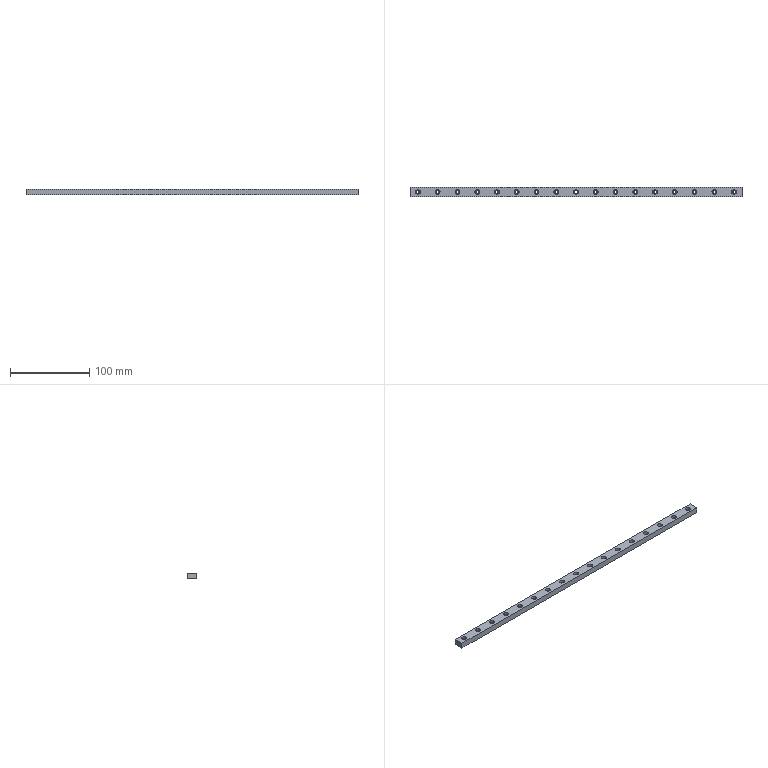Part | STEP file | BMC12B guide rail_L70 | 1 solid | 91 faces | box 420 x 12 x 7.5 mm | volume 35533 mm3 | cylinder 68 | plane 23 | commonest cylinder face diameters 3.4 x34 6 x34